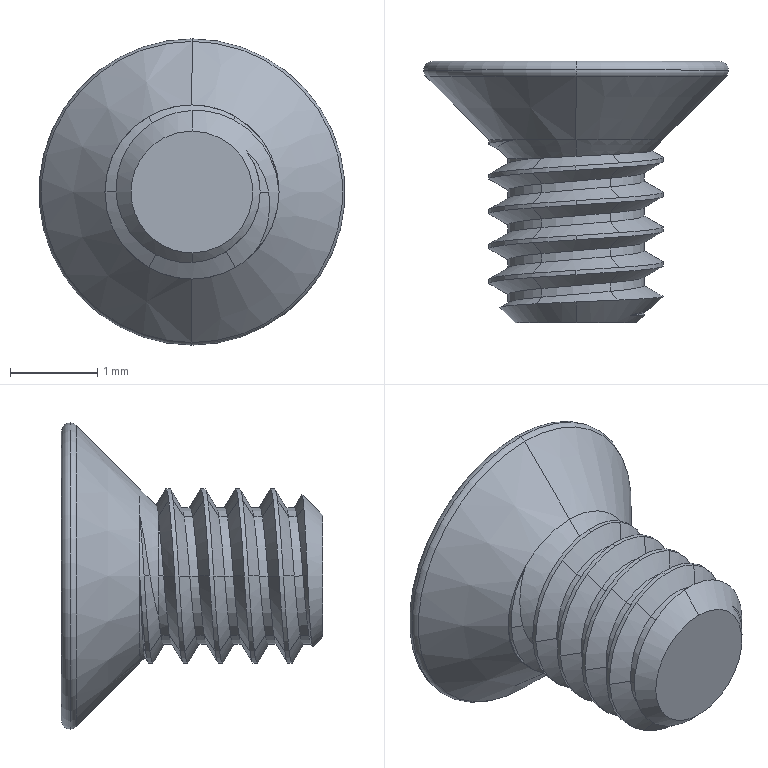Part | NX | features BREP 1 | 1 solid | 139 faces | box 3.517 x 3 x 3.517 mm | volume 9.817 mm3 | spline 65 | cylinder 47 | plane 15 | cone 8 | torus 4 | commonest cylinder face diameters 1.567 x29 2 x10 0.2 x8